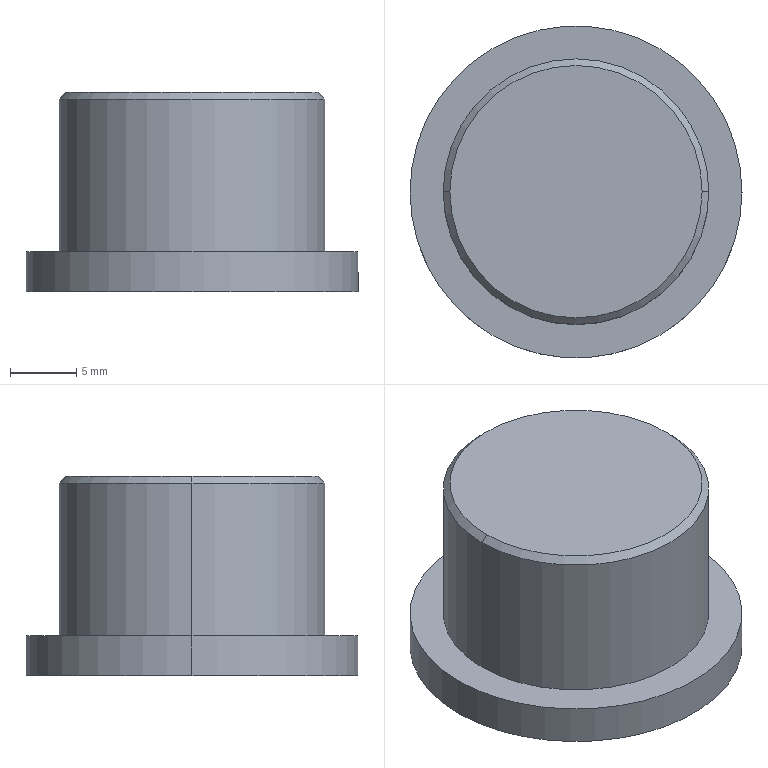Part | SolidWorks | features Chamfer 1, Revolution 1 | 1 solid | 9 faces | box 25 x 25 x 15 mm | volume 5235 mm3 | cylinder 4 | plane 3 | cone 2 | commonest cylinder face diameters 20 x2 25 x2
STEP:
#1=CARTESIAN_POINT('',(9.5,0.,0.));
#2=VERTEX_POINT('',#1);
#3=CARTESIAN_POINT('',(-9.5,0.,0.));
#4=VERTEX_POINT('',#3);
#5=CARTESIAN_POINT('',(0.,0.,0.));
#6=DIRECTION('',(0.,0.,1.));
#7=DIRECTION('',(-1.,0.,0.));
#8=AXIS2_PLACEMENT_3D('',#5,#6,#7);
#9=CIRCLE('',#8,9.5);
#10=EDGE_CURVE('',#2,#4,#9,.T.);
#11=ORIENTED_EDGE('',*,*,#10,.F.);
#12=CARTESIAN_POINT('',(10.,0.,-0.5));
#13=VERTEX_POINT('',#12);
#14=CARTESIAN_POINT('',(9.5,0.,0.));
#15=DIRECTION('',(0.7071,0.,-0.7071));
#16=VECTOR('',#15,1000.);
#17=LINE('',#14,#16);
#18=EDGE_CURVE('',#2,#13,#17,.T.);
#19=ORIENTED_EDGE('',*,*,#18,.T.);
#20=CARTESIAN_POINT('',(-10.,0.,-0.5));
#21=VERTEX_POINT('',#20);
#22=CARTESIAN_POINT('',(0.,0.,-0.5));
#23=DIRECTION('',(0.,0.,-1.));
#24=DIRECTION('',(-1.,0.,0.));
#25=AXIS2_PLACEMENT_3D('',#22,#23,#24);
#26=CIRCLE('',#25,10.);
#27=EDGE_CURVE('',#21,#13,#26,.T.);
#28=ORIENTED_EDGE('',*,*,#27,.F.);
#29=CARTESIAN_POINT('',(-9.5,0.,0.));
#30=DIRECTION('',(-0.7071,0.,-0.7071));
#31=VECTOR('',#30,1000.);
#32=LINE('',#29,#31);
#33=EDGE_CURVE('',#4,#21,#32,.T.);
#34=ORIENTED_EDGE('',*,*,#33,.F.);
#35=EDGE_LOOP('',(#11,#19,#28,#34));
#36=FACE_OUTER_BOUND('',#35,.T.);
#37=CARTESIAN_POINT('',(0.,0.,0.));
#38=DIRECTION('',(0.,0.,-1.));
#39=DIRECTION('',(-1.,0.,0.));
#40=AXIS2_PLACEMENT_3D('',#37,#38,#39);
#41=CONICAL_SURFACE('',#40,9.5,0.7854);
#42=ADVANCED_FACE('',(#36),#41,.T.);
#43=CARTESIAN_POINT('',(10.,0.,-12.));
#44=VERTEX_POINT('',#43);
#45=CARTESIAN_POINT('',(-10.,0.,-12.));
#46=VERTEX_POINT('',#45);
#47=CARTESIAN_POINT('',(0.,0.,-12.));
#48=DIRECTION('',(0.,0.,1.));
#49=DIRECTION('',(1.,0.,0.));
#50=AXIS2_PLACEMENT_3D('',#47,#48,#49);
#51=CIRCLE('',#50,10.);
#52=EDGE_CURVE('',#44,#46,#51,.T.);
#53=ORIENTED_EDGE('',*,*,#52,.T.);
#54=CARTESIAN_POINT('',(-10.,0.,0.));
#55=DIRECTION('',(0.,0.,1.));
#56=VECTOR('',#55,1000.);
#57=LINE('',#54,#56);
#58=EDGE_CURVE('',#46,#21,#57,.T.);
#59=ORIENTED_EDGE('',*,*,#58,.T.);
#60=ORIENTED_EDGE('',*,*,#27,.T.);
#61=CARTESIAN_POINT('',(10.,0.,0.));
#62=DIRECTION('',(0.,0.,1.));
#63=VECTOR('',#62,1000.);
#64=LINE('',#61,#63);
#65=EDGE_CURVE('',#44,#13,#64,.T.);
#66=ORIENTED_EDGE('',*,*,#65,.F.);
#67=EDGE_LOOP('',(#53,#59,#60,#66));
#68=FACE_OUTER_BOUND('',#67,.T.);
#69=CARTESIAN_POINT('',(0.,0.,0.));
#70=DIRECTION('',(0.,0.,1.));
#71=DIRECTION('',(1.,0.,0.));
#72=AXIS2_PLACEMENT_3D('',#69,#70,#71);
#73=CYLINDRICAL_SURFACE('',#72,10.);
#74=ADVANCED_FACE('',(#68),#73,.T.);
#75=CARTESIAN_POINT('',(12.5,0.,-15.));
#76=VERTEX_POINT('',#75);
#77=CARTESIAN_POINT('',(-12.5,0.,-15.));
#78=VERTEX_POINT('',#77);
#79=CARTESIAN_POINT('',(0.,0.,-15.));
#80=DIRECTION('',(0.,0.,1.));
#81=DIRECTION('',(1.,0.,0.));
#82=AXIS2_PLACEMENT_3D('',#79,#80,#81);
#83=CIRCLE('',#82,12.5);
#84=EDGE_CURVE('',#76,#78,#83,.T.);
#85=ORIENTED_EDGE('',*,*,#84,.T.);
#86=CARTESIAN_POINT('',(-12.5,0.,-12.));
#87=VERTEX_POINT('',#86);
#88=CARTESIAN_POINT('',(-12.5,0.,0.));
#89=DIRECTION('',(0.,0.,1.));
#90=VECTOR('',#89,1000.);
#91=LINE('',#88,#90);
#92=EDGE_CURVE('',#78,#87,#91,.T.);
#93=ORIENTED_EDGE('',*,*,#92,.T.);
#94=CARTESIAN_POINT('',(12.5,0.,-12.));
#95=VERTEX_POINT('',#94);
#96=CARTESIAN_POINT('',(0.,0.,-12.));
#97=DIRECTION('',(0.,0.,1.));
#98=DIRECTION('',(1.,0.,0.));
#99=AXIS2_PLACEMENT_3D('',#96,#97,#98);
#100=CIRCLE('',#99,12.5);
#101=EDGE_CURVE('',#95,#87,#100,.T.);
#102=ORIENTED_EDGE('',*,*,#101,.F.);
#103=CARTESIAN_POINT('',(12.5,0.,0.));
#104=DIRECTION('',(0.,0.,1.));
#105=VECTOR('',#104,1000.);
#106=LINE('',#103,#105);
#107=EDGE_CURVE('',#76,#95,#106,.T.);
#108=ORIENTED_EDGE('',*,*,#107,.F.);
#109=EDGE_LOOP('',(#85,#93,#102,#108));
#110=FACE_OUTER_BOUND('',#109,.T.);
#111=CARTESIAN_POINT('',(0.,0.,0.));
#112=DIRECTION('',(0.,0.,1.));
#113=DIRECTION('',(1.,0.,0.));
#114=AXIS2_PLACEMENT_3D('',#111,#112,#113);
#115=CYLINDRICAL_SURFACE('',#114,12.5);
#116=ADVANCED_FACE('',(#110),#115,.T.);
#117=ORIENTED_EDGE('',*,*,#84,.F.);
#118=CARTESIAN_POINT('',(0.,0.,-15.));
#119=DIRECTION('',(0.,0.,1.));
#120=DIRECTION('',(1.,0.,0.));
#121=AXIS2_PLACEMENT_3D('',#118,#119,#120);
#122=CIRCLE('',#121,12.5);
#123=EDGE_CURVE('',#78,#76,#122,.T.);
#124=ORIENTED_EDGE('',*,*,#123,.F.);
#125=EDGE_LOOP('',(#117,#124));
#126=FACE_OUTER_BOUND('',#125,.T.);
#127=CARTESIAN_POINT('',(0.,0.,-15.));
#128=DIRECTION('',(0.,0.,1.));
#129=DIRECTION('',(1.,0.,0.));
#130=AXIS2_PLACEMENT_3D('',#127,#128,#129);
#131=PLANE('',#130);
#132=ADVANCED_FACE('',(#126),#131,.F.);
#133=ORIENTED_EDGE('',*,*,#92,.F.);
#134=ORIENTED_EDGE('',*,*,#123,.T.);
#135=ORIENTED_EDGE('',*,*,#107,.T.);
#136=CARTESIAN_POINT('',(0.,0.,-12.));
#137=DIRECTION('',(0.,0.,1.));
#138=DIRECTION('',(1.,0.,0.));
#139=AXIS2_PLACEMENT_3D('',#136,#137,#138);
#140=CIRCLE('',#139,12.5);
#141=EDGE_CURVE('',#87,#95,#140,.T.);
#142=ORIENTED_EDGE('',*,*,#141,.F.);
#143=EDGE_LOOP('',(#133,#134,#135,#142));
#144=FACE_OUTER_BOUND('',#143,.T.);
#145=CARTESIAN_POINT('',(0.,0.,0.));
#146=DIRECTION('',(0.,0.,1.));
#147=DIRECTION('',(1.,0.,0.));
#148=AXIS2_PLACEMENT_3D('',#145,#146,#147);
#149=CYLINDRICAL_SURFACE('',#148,12.5);
#150=ADVANCED_FACE('',(#144),#149,.T.);
#151=ORIENTED_EDGE('',*,*,#52,.F.);
#152=CARTESIAN_POINT('',(0.,0.,-12.));
#153=DIRECTION('',(0.,0.,1.));
#154=DIRECTION('',(1.,0.,0.));
#155=AXIS2_PLACEMENT_3D('',#152,#153,#154);
#156=CIRCLE('',#155,10.);
#157=EDGE_CURVE('',#46,#44,#156,.T.);
#158=ORIENTED_EDGE('',*,*,#157,.F.);
#159=EDGE_LOOP('',(#151,#158));
#160=FACE_BOUND('',#159,.T.);
#161=ORIENTED_EDGE('',*,*,#101,.T.);
#162=ORIENTED_EDGE('',*,*,#141,.T.);
#163=EDGE_LOOP('',(#161,#162));
#164=FACE_OUTER_BOUND('',#163,.T.);
#165=CARTESIAN_POINT('',(0.,12.5,-12.));
#166=DIRECTION('',(0.,0.,-1.));
#167=DIRECTION('',(-1.,0.,0.));
#168=AXIS2_PLACEMENT_3D('',#165,#166,#167);
#169=PLANE('',#168);
#170=ADVANCED_FACE('',(#160,#164),#169,.F.);
#171=ORIENTED_EDGE('',*,*,#58,.F.);
#172=ORIENTED_EDGE('',*,*,#157,.T.);
#173=ORIENTED_EDGE('',*,*,#65,.T.);
#174=CARTESIAN_POINT('',(0.,0.,-0.5));
#175=DIRECTION('',(0.,0.,-1.));
#176=DIRECTION('',(-1.,0.,0.));
#177=AXIS2_PLACEMENT_3D('',#174,#175,#176);
#178=CIRCLE('',#177,10.);
#179=EDGE_CURVE('',#13,#21,#178,.T.);
#180=ORIENTED_EDGE('',*,*,#179,.T.);
#181=EDGE_LOOP('',(#171,#172,#173,#180));
#182=FACE_OUTER_BOUND('',#181,.T.);
#183=CARTESIAN_POINT('',(0.,0.,0.));
#184=DIRECTION('',(0.,0.,1.));
#185=DIRECTION('',(1.,0.,0.));
#186=AXIS2_PLACEMENT_3D('',#183,#184,#185);
#187=CYLINDRICAL_SURFACE('',#186,10.);
#188=ADVANCED_FACE('',(#182),#187,.T.);
#189=CARTESIAN_POINT('',(0.,0.,0.));
#190=DIRECTION('',(0.,0.,1.));
#191=DIRECTION('',(-1.,0.,0.));
#192=AXIS2_PLACEMENT_3D('',#189,#190,#191);
#193=CIRCLE('',#192,9.5);
#194=EDGE_CURVE('',#4,#2,#193,.T.);
#195=ORIENTED_EDGE('',*,*,#194,.T.);
#196=ORIENTED_EDGE('',*,*,#10,.T.);
#197=EDGE_LOOP('',(#195,#196));
#198=FACE_OUTER_BOUND('',#197,.T.);
#199=CARTESIAN_POINT('',(0.,10.,0.));
#200=DIRECTION('',(0.,0.,-1.));
#201=DIRECTION('',(-1.,0.,0.));
#202=AXIS2_PLACEMENT_3D('',#199,#200,#201);
#203=PLANE('',#202);
#204=ADVANCED_FACE('',(#198),#203,.F.);
#205=ORIENTED_EDGE('',*,*,#18,.F.);
#206=ORIENTED_EDGE('',*,*,#194,.F.);
#207=ORIENTED_EDGE('',*,*,#33,.T.);
#208=ORIENTED_EDGE('',*,*,#179,.F.);
#209=EDGE_LOOP('',(#205,#206,#207,#208));
#210=FACE_OUTER_BOUND('',#209,.T.);
#211=CARTESIAN_POINT('',(0.,0.,0.));
#212=DIRECTION('',(0.,0.,-1.));
#213=DIRECTION('',(-1.,0.,0.));
#214=AXIS2_PLACEMENT_3D('',#211,#212,#213);
#215=CONICAL_SURFACE('',#214,9.5,0.7854);
#216=ADVANCED_FACE('',(#210),#215,.T.);
#217=CLOSED_SHELL('',(#42,#74,#116,#132,#150,#170,#188,#204,#216));
#218=MANIFOLD_SOLID_BREP('',#217);
#219=CARTESIAN_POINT('',(0.,0.,0.));
#220=DIRECTION('',(0.,0.,1.));
#221=DIRECTION('',(1.,0.,0.));
#222=AXIS2_PLACEMENT_3D('',#219,#220,#221);
#223=(LENGTH_UNIT()NAMED_UNIT(*)SI_UNIT(.MILLI.,.METRE.));
#224=UNCERTAINTY_MEASURE_WITH_UNIT(LENGTH_MEASURE(0.00001),#223,'','');
#225=(NAMED_UNIT(*)PLANE_ANGLE_UNIT()SI_UNIT($,.RADIAN.));
#226=(NAMED_UNIT(*)SI_UNIT($,.STERADIAN.)SOLID_ANGLE_UNIT());
#227=(GEOMETRIC_REPRESENTATION_CONTEXT(3)GLOBAL_UNCERTAINTY_ASSIGNED_CONTEXT((#224))GLOBAL_UNIT_ASSIGNED_CONTEXT((#223,#225,#226))REPRESENTATION_CONTEXT('',''));
#228=ADVANCED_BREP_SHAPE_REPRESENTATION('',(#218,#222),#227);